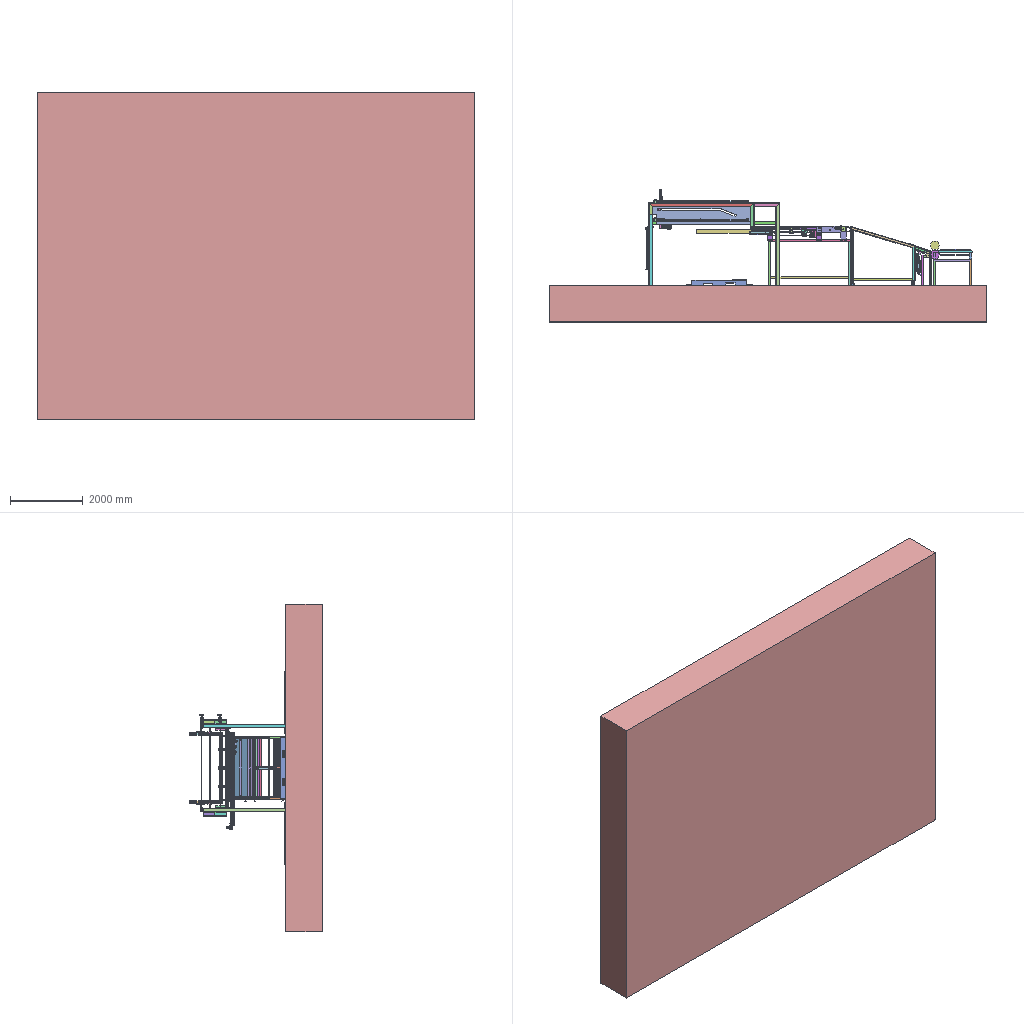Assembly | STEP file | 259 different items | 1357 placed | box 12000 x 3640 x 9000 mm
Parts list (item | name | quantity | parent item | size | volume):
1 | 200W right-angle motor | x3 | in Chuan-type roller line | 116.75 x 104.5 x 320.75 mm | 2722546 mm3
2 | 40 x 40 x 1200-2 | x2 | in FZC-000-001 Upper 1 | 40 x 40 x 1520 mm | 812891 mm3
3 | 40 x 40 x 1700 | x1 | in FZC-000-001 Upper 1 | 40 x 40 x 1620 mm | 866370 mm3
4 | 40 x 40 x 200 | x2 | in FZC-000-001 Upper 1 | 40 x 40 x 98 mm | 52410 mm3
5 | 40 x 40 x 920 | x2 | in FZC-000-001 Upper 1 | 40 x 40 x 1480 mm | 791499 mm3
6 | 40 x 60 x 710 -2_Default<Machined> | x2 | in FZC-000-001 Upper 1 | 710 x 40 x 60 mm | 494666 mm3
7 | 40 x 60 x 940_Default<Machined> | x2 | in FZC-000-001 Upper 1, TN-NHGJQJ-001 | 940 x 40 x 60 mm | 663437 mm3
8 | 40X35X65 oil-free bushing | x4 | in Hydraulic lifting platform assembly | 40 x 40 x 65 mm | 19085 mm3
9 | - | x1 | in MFBR060-L1-14-50-70-M4-33.STEP.STEP_3.STEP_1.STEP_2.STEP.STEP | 29 x 65.5 x 65.5 mm | 78909 mm3
10 | Aluminium profile frame 2_Default<Machined> | x1 | in Sheet stacking line | 2080 x 80 x 40 mm | 1541424 mm3
11 | Aluminium profile frame_Default<Machined> | x1 | in Sheet stacking line | 1808 x 80 x 40 mm | 1339853 mm3
12 | Anti-vibration sleeve | x1 | in Telescopic belt | 173 x 110 x 10 mm | 116462 mm3
13 | BABR060_X2_8f9351658f74_X0_-14.STEP | x1 | in MFBR060-L2-14-50-70-M5-33.STEP | 20 x 20 x 29 mm | 3932 mm3
14 | - | x6 | in GRM4TS-6-75-75-LAA-B10-CLOSED | 156.007 x 55.626 x 50.292 mm | 208315 mm3
15 | BT2022003-01-04 Pin shaft A | x4 | in Hydraulic lifting platform assembly | 109.5 x 31 x 31 mm | 54297 mm3
16 | BT2022003-01-05 Scissor beam A_Default<Machined> | x1 | in Hydraulic lifting platform assembly | 1300 x 120 x 1590 mm | 10641393 mm3
17 | BT2022003-01-06 Scissor beam B_Default<Machined> | x1 | in Hydraulic lifting platform assembly | 1311 x 120 x 1590 mm | 5354127 mm3
18 | BT2022003-01-09 Pin shaft C | x4 | in Hydraulic lifting platform assembly | 125 x 42 x 42 mm | 110638 mm3
19 | BT2022003-01-10 Guide wheel A | x2 | in Hydraulic lifting platform assembly | 26 x 106 x 106 mm | 151941 mm3
20 | BT2022003-10 Liner plate | x4 | in Hydraulic lifting platform assembly | 500 x 4 x 50 mm | 96702 mm3
21 | Baffle 3 | x5 | in Sheet stacking line | 2070 x 50 x 90 mm | 281521 mm3
22 | Base plate 1_Default<Machined> | x1 | in Flip clamping mechanism | 140 x 180 x 12 mm | 295903 mm3
23 | Base plate 2_Default<Machined> | x1 | in Flip clamping mechanism | 40 x 180 x 12 mm | 81882 mm3
24 | Base_Default<Machined> | x1 | in Sheet stacking line | 840 x 60 x 1700 mm | 2443992 mm3
25 | Bearing housing 1 | x3 | in Telescopic belt | 97 x 97 x 35 mm | 155576 mm3
26 | Bearing housing 2 | x3 | in Bearing housing 2 assembly | 114 x 62 x 31 mm | 91139 mm3
27 | Belt | x1 | in Sheet stacking line | 2560 x 1600 x 60 mm | 33125947 mm3
28 | Bracket_Default<Machined> | x2 | in Sheet stacking line | 3700 x 200 x 2275 mm | 12653736 mm3
29 | Connecting plate | x3 | in Telescopic belt | 150 x 240 x 12 mm | 410487 mm3
30 | Conveyor belt | x1 | in Telescopic belt | 2753 x 173 x 1600 mm | 42849624 mm3
31 | Conveyor line bracket_Default<Machined> | x1 | in Sheet stacking line | 1782 x 1478 x 1726 mm | 68319055 mm3
32 | Cross beam 2_Default<Machined> | x2 | in Sheet stacking line | 3400 x 100 x 180 mm | 5412412 mm3
33 | Cross beam_Default<Machined> | x1 | in Sheet stacking line | 2220 x 107.726 x 177.73 mm | 3150772 mm3
34 | DCL01-D40-B-d16-e16 | x1 | in Flip clamping mechanism | 40 x 40 x 66 mm | 65701 mm3
35 | Drive belt | x1 | in Telescopic belt | 332.993 x 128 x 25 mm | 76914 mm3
36 | Drive shaft | x6 | in Chuan-type roller line | 870 x 25 x 25 mm | 420131 mm3
37 | Driving pulley | x4 | in Telescopic belt | 65.94 x 65.413 x 30 mm | 79962 mm3
38 | Driving shaft key | x1 | in Telescopic belt | 30 x 8 x 7 mm | 1584 mm3
39 | EE_SX951P_W | x2 | in Flip clamping mechanism | 13.4 x 12 x 22 mm | 1092 mm3
40 | Edge guard | x6 | in Chuan-type roller line | 35 x 25 x 1700 mm | 453852 mm3
41 | Elastic block | x6 | in Telescopic belt | 24 x 24 x 25 mm | 8627 mm3
42 | End strip | x2 | in Telescopic belt | 10 x 10 x 432 mm | 42976 mm3
43 | FZC-000-002 Rotating shaft A | x4 | in FZC-000-001 Upper 1, Sheet stacking line | 40 x 50 x 100 mm | 133744 mm3
44 | FZC-000-003 Upper cylinder support | x6 | in FZC-000-001 Upper 1, Sheet stacking line | 100 x 60 x 70 mm | 117991 mm3
45 | Fixing block | x2 | in Middle section assembly, Telescopic belt | 105 x 80 x 80 mm | 486425 mm3
46 | Flip baffle_Default<Machined> | x1 | in Sheet stacking line | 1040 x 45 x 1590 mm | 10479554 mm3
47 | Frame 1_Default<Machined> | x2 | in Final assembly | 1700 x 320 x 60 mm | 1222260 mm3
48 | GB893.2-86 internal retaining ring type B 62 | x4 | in Hydraulic lifting platform assembly | 66.2 x 64.58 x 2 mm | 1598 mm3
49 | GB894.2-86 shaft retaining ring type B 25 | x4 | in Hydraulic lifting platform assembly | 28.2 x 30.934 x 1.2 mm | 273.026 mm3
50 | GB894.2-86 shaft retaining ring type B 30 | x4 | in Hydraulic lifting platform assembly | 33.5 x 36.623 x 1.2 mm | 375.357 mm3
51 | GB/T276-94 deep groove ball bearing 6206-2Z | x4 | in Hydraulic lifting platform assembly | 16 x 62 x 62 mm | 23194 mm3
52 | GB/T41-20001 hex nut grade C M12 | x2 | in Sheet stacking line | 19.85 x 17.191 x 12.2 mm | 1737 mm3
53 | GB/T6172.1-2000 hex thin nut grade A and B (M27) | x8 | in Hydraulic lifting platform assembly | 39.233 x 45.2 x 13.5 mm | 9913 mm3
54 | GB/T6172.1-2000 hex thin nut grade A and B M30 | x4 | in Hydraulic lifting platform assembly | 44.137 x 50.85 x 15 mm | 14200 mm3
55 | GDT40-2000 | x3 | in Chuan-type roller line | 20 x 10 x 1400 mm | 237664 mm3
56 | GRM4_B10_BODYOPTION_M | x6 | in GRM4TS-6-75-75-LAA-B10-CLOSED | 50.292 x 55.27 x 73.66 mm | 161375 mm3
57 | GRM4_B10_TUBE_M_71195-001-002100 | x6 | in GRM4TS-6-75-75-LAA-B10-CLOSED | 53.34 x 6.35 x 6.35 mm | 997.325 mm3
58 | GRM4_BREATHER_VENT_71996_M | x6 | in GRM4TS-6-75-75-LAA-B10-CLOSED | 14 x 13 x 15.011 mm | 1457 mm3
59 | GRM4_IMP_PLATE_64636-02_M | x12 | in GRM4TS-6-75-75-LAA-B10-CLOSED | 101.954 x 130.048 x 2.667 mm | 13683 mm3
60 | Gripper baffle | x2 | in Sheet stacking line | 1420 x 5 x 50 mm | 355000 mm3
61 | Ground | x1 | in Sheet stacking line | 12000 x 1000 x 9000 mm | 101165700000 mm3
62 | Guard plate | x144 | in Chuan-type roller line | 328 x 3 x 50 mm | 48733 mm3
63 | Guide rail sliding pair | x3 | in Middle section assembly, Telescopic belt | 63 x 74 x 26.5 mm | 70725 mm3
64 | HB362-65 end not tightened, ground flat 0.25 turns 15×50 | x2 | in Sheet stacking line | 17 x 17 x 50.4 mm | 1550 mm3
65 | HGH20_3_AF0 | x2 | in Sheet stacking line | 44 x 25.4 x 77.5 mm | 65768 mm3
66 | HGR20_3_AF0 | x1 | in Sheet stacking line | 20 x 17.5 x 900 mm | 257708 mm3
67 | HI_BMH070 Flansch | x2 | in Frame-type span dual-rail module | 48.5 x 70.1 x 70 mm | 191060 mm3
68 | Head plate 1 | x1 | in Telescopic belt | 810 x 379.049 x 14 mm | 2266923 mm3
69 | Head plate 2 | x1 | in Telescopic belt | 810 x 160 x 14 mm | 1785161 mm3
70 | Hydraulic cylinder A-400 | x5 | in Final assembly, Sheet stacking line | 60 x 60 x 540 mm | 1442964 mm3
71 | Hydraulic cylinder B-500 | x5 | in Final assembly, Sheet stacking line | 30 x 30 x 411 mm | 278111 mm3
72 | Hydraulic cylinder body SLDPRT | x2 | in 95x80x40x400 hydraulic cylinder assembly | 127.5 x 520 x 95 mm | 2648079 mm3
73 | Idler roller shaft | x1 | in Telescopic belt | 35 x 35 x 408 mm | 356727 mm3
74 | Inner slide strip | x2 | in Telescopic belt | 20 x 20 x 520 mm | 207468 mm3
75 | JB/T7940.1-1995 straight-through grease cup 6 | x2 | in Hydraulic lifting platform assembly | 8 x 13 x 9.238 mm | 360.504 mm3
76 | KFL005 | x6 | in Chuan-type roller line | 60 x 100 x 24.5 mm | 44047 mm3
77 | Key 2 | x1 | in Telescopic belt | 40 x 12 x 8 mm | 3593 mm3
78 | L40 angle steel | x3 | in Telescopic belt | 40 x 40 x 20 mm | 4347 mm3
79 | LEB23-20 | x5 | in Manual lead screw mechanism | 95 x 58 x 61 mm | 169444 mm3
80 | LEB31-20 | x5 | in Manual lead screw mechanism | 95 x 58 x 26 mm | 76469 mm3
81 | Large pulley | x1 | in Telescopic belt | 120.932 x 120.932 x 40 mm | 261557 mm3
82 | Linear motion ball bearing | x4 | in Telescopic belt | 44 x 44 x 44 mm | 35802 mm3
83 | M4_4.STEP_1.STEP_2.STEP.STEP | x4 | in MFBR060-L1-14-50-70-M4-33.STEP_7.STEP_2.STEP.STEP | 24 x 7 x 7 mm | 386.258 mm3
84 | M5.STEP | x1 | in MFBR060-L2-14-50-70-M5-33.STEP | 25 x 8.5 x 8.5 mm | 634.487 mm3
85 | MET_JAW_STD_ROT_GRM4 | x12 | in GRM4TS-6-75-75-LAA-B10-CLOSED | 152.146 x 76.2 x 25.425 mm | 65062 mm3
86 | Main motor | x1 | in Telescopic belt | 120 x 120 x 170 mm | 887990 mm3
87 | Middle plate 1 | x1 | in Telescopic belt | 1500 x 400 x 84 mm | 3461326 mm3
88 | Middle plate 2 | x1 | in Middle section assembly | 1500 x 400 x 84 mm | 3459743 mm3
89 | Mirror HGH20_3_AF0 | x2 | in Sheet stacking line | 44 x 25.4 x 77.5 mm | 65768 mm3
90 | Mirror HGR20_3_AF0 | x1 | in Sheet stacking line | 20 x 17.5 x 900 mm | 257708 mm3
91 | Mirror rail shaft | x1 | in Sheet stacking line | 2134 x 75 x 100 mm | 1735049 mm3
92 | Mirror rail_Default<Machined> | x1 | in Sheet stacking line | 2900 x 115 x 650 mm | 29036229 mm3
93 | Mirror slide plate 2 | x1 | in Sheet stacking line | 90 x 148.62 x 100 mm | 228620 mm3
94 | Mirror slide plate 3 | x1 | in Sheet stacking line | 196 x 218.322 x 100 mm | 404322 mm3
95 | Mirror slider 12 | x1 | in Sheet stacking line | 60 x 60 x 350 mm | 385000 mm3
96 | Mirror slider 13 | x1 | in Sheet stacking line | 60 x 60 x 900 mm | 990000 mm3
97 | Motor bracket | x1 | in Flip clamping mechanism | 65 x 68 x 110 mm | 111617 mm3
98 | Motor mounting plate | x1 | in Telescopic belt | 310 x 180 x 20 mm | 521549 mm3
99 | OT2025004-02-10 Shaft 2 | x1 | in Flip clamping mechanism | 25 x 946 x 25 mm | 439586 mm3
100 | Open CASCADE STEP translator 7.6 56.2.1.1 | x5 | in Open CASCADE STEP translator | 130.4 x 85.907 x 80 mm | 551180 mm3
101 | Open CASCADE STEP translator 7.6 56.2.1.2 | x5 | in Open CASCADE STEP translator | 37.25 x 32.25 x 30.8 mm | 9079 mm3
102 | Open CASCADE STEP translator 7.6 56.2.1.3 | x5 | in Open CASCADE STEP translator | 7.6 x 40.2 x 7.6 mm | 1264 mm3
103 | Open CASCADE STEP translator 7.6 56.2.1.4 | x5 | in Open CASCADE STEP translator | 14.55 x 23.7 x 11.2 mm | 1255 mm3
104 | Open CASCADE STEP translator 7.6 56.2.1.5 | x5 | in Open CASCADE STEP translator | 12.626 x 16.806 x 25 mm | 1310 mm3
105 | Open CASCADE STEP translator 7.6 56.2.1.6 | x5 | in Open CASCADE STEP translator | 6 x 36.756 x 6 mm | 671.876 mm3
106 | Open CASCADE STEP translator 7.6 56.2.1.7 | x5 | in Open CASCADE STEP translator | 19 x 23.7 x 14.5 mm | 1788 mm3
107 | PN59104-114_M_SHCSM6x1x10 | x36 | in GRM4TS-6-75-75-LAA-B10-CLOSED | 10 x 16 x 10 mm | 680.296 mm3
108 | PN59104-141_M_SHCSM8x1.25x25 | x18 | in GRM4TS-6-75-75-LAA-B10-CLOSED | 13 x 33 x 13 mm | 2174 mm3
109 | PN62195-005_METRIC_PLASTIC_TUBE_FITTING | x24 | in GRM4TS-6-75-75-LAA-B10-CLOSED | 26 x 26.85 x 13.856 mm | 3050 mm3
110 | PN_0001-01-01 Lifting platform top cover_Default<Machined> | x1 | in Hydraulic lifting platform assembly | 1500 x 195 x 1800 mm | 133503358 mm3
111 | PN_0001-01-02 Lifting platform base_Default<Machined> | x1 | in Hydraulic lifting platform assembly | 1480 x 1665 x 80 mm | 7503788 mm3
112 | PN_0001-01-07 Pin shaft B | x2 | in Hydraulic lifting platform assembly | 175 x 48.5 x 48.5 mm | 160152 mm3
113 | PN_0001-01-08 Pad | x2 | in Hydraulic lifting platform assembly | 55 x 55 x 5 mm | 8159 mm3
114 | PN_0001-01-11 Guide wheel B | x2 | in Hydraulic lifting platform assembly | 29 x 90 x 90 mm | 98573 mm3
115 | PN_0001-01-12 Sensor board | x1 | in Hydraulic lifting platform assembly | 66 x 58.5 x 2 mm | 7091 mm3
116 | PN_0001-11 Cover plate A | x1 | in Hydraulic lifting platform assembly | 312 x 240 x 3 mm | 222709 mm3
117 | PN_0001-12 Cover plate B | x2 | in Hydraulic lifting platform assembly | 180 x 150 x 340 mm | 329639 mm3
118 | Pad plate | x1 | in FZC-000-001 Upper 1 | 1700 x 1520 x 2 mm | 5168000 mm3
119 | Part 32 | x2 | in Sheet stacking line | 100 x 60 x 40 mm | 240000 mm3
120 | Part 38_Default<Machined> | x1 | in Sheet stacking line | 1720 x 2260 x 1280 mm | 9110278 mm3
121 | Piston rod | x2 | in 95x80x40x400 hydraulic cylinder assembly | 430 x 80 x 80 mm | 691930 mm3
122 | Plain washers-N series-Grade1 A GB_GB_FASTENER_WASHER_PWNA 20 | x3 | in Telescopic belt | 37 x 37 x 3 mm | 2187 mm3
123 | Plate 2 | x6 | in Sheet stacking line | 350 x 5 x 1500 mm | 2625000 mm3
124 | Pressure plate | x7 | in Telescopic belt | 30 x 30 x 6 mm | 3958 mm3
125 | Pressure plate 2 | x66 | in Sheet stacking line | 50 x 6 x 30 mm | 6094 mm3
126 | Pressure plate 3 | x4 | in Sheet stacking line | 1420 x 20 x 30 mm | 852000 mm3
127 | Profile 4060100 | x5 | in TN-NHGJQJ-001 | 40 x 60 x 99.7 mm | 57095 mm3
128 | Profile 40601120 | x1 | in FZC-000-001 Upper 1 | 40 x 60 x 1120 mm | 641390 mm3
129 | Profile 40601200-1 | x4 | in FZC-000-001 Upper 1, TN-NHGJQJ-001 | 40 x 60 x 1200 mm | 664297 mm3
130 | Profile 40601620 | x3 | in FZC-000-001 Upper 1, TN-NHGJQJ-001 | 40 x 60 x 1620 mm | 927725 mm3
131 | Profile 40601700 | x4 | in FZC-000-001 Upper 1, TN-NHGJQJ-001 | 40 x 60 x 1700 mm | 950632 mm3
132 | Profile 4060920 | x2 | in TN-NHGJQJ-001 | 40 x 60 x 920 mm | 526856 mm3
133 | Rail shaft | x1 | in Sheet stacking line | 2134 x 75 x 100 mm | 1735049 mm3
134 | Rail_Default<Machined> | x1 | in Sheet stacking line | 2900 x 115 x 650 mm | 29036229 mm3
135 | Reducer | x1 | in Telescopic belt | 130 x 170 x 120 mm | 1507884 mm3
136 | Retracting rod | x3 | in Telescopic belt | 30 x 30 x 1045 mm | 737225 mm3
137 | Roller 1 | x1 | in Telescopic belt | 120 x 120 x 570 mm | 928585 mm3
138 | Roller 11 | x1 | in Sheet stacking line | 50 x 1800 x 50 mm | 3218952 mm3
139 | Roller 2 | x4 | in Telescopic belt | 50 x 50 x 350 mm | 233051 mm3
140 | Roller line_Default<Machined> | x1 | in Sheet stacking line | 1152 x 1230 x 1771 mm | 196274753 mm3
141 | Roller sheet metal | x3 | in Chuan-type roller line | 380 x 110 x 1700 mm | 4838420 mm3
142 | Roller sheet metal_Mirror Default | x3 | in Chuan-type roller line | 380 x 110 x 1700 mm | 4838420 mm3
143 | Sensor detection tab | x1 | in Flip clamping mechanism | 20 x 18 x 10 mm | 512.842 mm3
144 | Shaft 2 | x1 | in Telescopic belt | 35 x 35 x 550 mm | 418334 mm3
145 | Shaft 3 | x1 | in Telescopic belt | 35 x 35 x 448 mm | 375515 mm3
146 | Shaft 4 | x2 | in Telescopic belt | 35 x 35 x 470 mm | 385852 mm3
147 | Sheath | x1 | in Telescopic belt | 25.34 x 28.859 x 45 mm | 22979 mm3
148 | Sheet metal 11 | x3 | in Chuan-type roller line | 350 x 75 x 1700 mm | 3328088 mm3
149 | Sheet metal 12 | x6 | in Chuan-type roller line | 245 x 75 x 1620 mm | 2491073 mm3
150 | Short conveyor line_Default<Machined> | x1 | in Sheet stacking line | 474.996 x 192.498 x 1720 mm | 30115690 mm3
151 | Single sprocket roller_08B | x96 | in Chuan-type roller line | 365.5 x 65.419 x 65.772 mm | 961298 mm3
152 | Sleeve | x27 | in Chuan-type roller line | 130 x 60 x 60 mm | 302189 mm3
153 | Slide plate 2 | x1 | in Sheet stacking line | 90 x 148.62 x 100 mm | 228620 mm3
154 | Slide plate 3 | x1 | in Sheet stacking line | 196 x 218.322 x 100 mm | 404322 mm3
155 | Slide rod | x3 | in Middle section assembly, Telescopic belt | 640 x 20 x 17.5 mm | 214573 mm3
156 | Slider | x3 | in Middle section assembly, Telescopic belt | 100 x 155 x 60 mm | 283785 mm3
157 | Slider 12 | x1 | in Sheet stacking line | 60 x 60 x 350 mm | 385000 mm3
158 | Slider 13 | x1 | in Sheet stacking line | 60 x 60 x 900 mm | 990000 mm3
159 | Slider pressure plate | x3 | in Slider pressure plate assembly | 100 x 60 x 8 mm | 42576 mm3
160 | Small pulley | x1 | in Telescopic belt | 59.476 x 59.476 x 25 mm | 54452 mm3
161 | Spacer block | x4 | in Telescopic belt | 20 x 20 x 54 mm | 21404 mm3
162 | Spacer block 22 | x10 | in Sheet stacking line | 95 x 40 x 40 mm | 152000 mm3
163 | Spring lock washers--Normal1 type GB_GB_FASTENER_WASHER_SW 20 | x3 | in Telescopic belt | 31.04 x 31.04 x 5 mm | 1973 mm3
164 | Square block | x3 | in Telescopic belt | 60 x 50 x 50 mm | 104625 mm3
165 | Square tube | x1 | in Telescopic belt | 80 x 80 x 80 mm | 136796 mm3
166 | Stopper | x6 | in Stopper assembly | 50 x 50 x 35 mm | 78331 mm3
167 | Stopper rack 12_Default<Machined> | x1 | in Sheet stacking line | 1700 x 164 x 1145 mm | 2370796 mm3
168 | Stopper rack_Default<Machined> | x1 | in Sheet stacking line | 575 x 40 x 2540 mm | 2334872 mm3
169 | Stud | x2 | in Sheet stacking line | 12 x 120 x 12 mm | 13572 mm3
170 | Support rod | x1 | in Telescopic belt | 20 x 20 x 408 mm | 162668 mm3
171 | Support rod 2 | x3 | in Telescopic belt | 20 x 20 x 380 mm | 150404 mm3
172 | Support sheet metal | x126 | in Chuan-type roller line | 112 x 70 x 20 mm | 9602 mm3
173 | Synchronous driving pulley key | x2 | in Telescopic belt | 20 x 5 x 5 mm | 473.175 mm3
174 | Synchronous key | x1 | in Telescopic belt | 25 x 8 x 7 mm | 1400 mm3
175 | Synchronous motor | x1 | in Telescopic belt | 130 x 130 x 239 mm | 1553555 mm3
176 | Synchronous shaft 1 | x3 | in Telescopic belt | 25 x 25 x 89 mm | 25420 mm3
177 | Synchronous shaft 2 | x2 | in Telescopic belt | 40 x 40 x 486 mm | 415215 mm3
178 | T-BDJ-204 | x2 | in Flip clamping mechanism | 37 x 65 x 127 mm | 102514 mm3
179 | TN-NHGJQJ-001-001 | x4 | in Sheet stacking line, TN-NHGJQJ-001 | 150 x 40 x 55 mm | 96398 mm3
180 | TN-NHGJQJ-001-002 | x6 | in Sheet stacking line, TN-NHGJQJ-001 | 100 x 120 x 110 mm | 222546 mm3
181 | Telescopic plate | x1 | in Telescopic belt | 296 x 35 x 1190 mm | 1170000 mm3
182 | Thin steel plate | x1 | in Telescopic belt | 350 x 1 x 1590 mm | 556500 mm3
183 | Timing belt | x3 | in Telescopic belt | 1001 x 71 x 25 mm | 155522 mm3
184 | Timing pulley | x2 | in Telescopic belt | 65.94 x 65.413 x 30 mm | 80276 mm3
185 | Tray | x1 | in Sheet stacking line | 1500 x 150 x 1700 mm | 287460631 mm3
186 | Underframe_Default<Machined> | x1 | in Sheet stacking line | 1740 x 260 x 970 mm | 7091962 mm3
187 | Unpowered roller | x48 | in Chuan-type roller line | 334.5 x 60 x 60 mm | 930239 mm3
188 | X2MH010A-N2C (connector type) -1 | x1 | in Flip clamping mechanism | 40 x 54.95 x 96 mm | 118411 mm3
189 | YBLX-ME-8108 limit switch | x1 | in Hydraulic lifting platform assembly | 28.5 x 180 x 50 mm | 106221 mm3
190 | _1-LCV02-25-5-L1400-F27-P101 | x5 | in Manual lead screw mechanism | 25 x 25 x 2604 mm | 1237665 mm3
191 | _2-LCV02-25-5-L1400-F27-P102 | x5 | in Manual lead screw mechanism, Sheet stacking line | 48 x 62 x 51 mm | 50671 mm3
192 | _Achsprofil-SBG - PAS42 B 1236 | x4 | in Frame-type span dual-rail module | 2456 x 60 x 60 mm | 8161158 mm3
193 | _BMH070 Abschlussdeckel | x2 | in Frame-type span dual-rail module | 8 x 70 x 70 mm | 28903 mm3
194 | _BMH070 Lagerschild2A154 | x2 | in Frame-type span dual-rail module | 100 x 70.1 x 70 mm | 431023 mm3
195 | _BMH070 Signalstecker gerade1 | x2 | in Frame-type span dual-rail module | 51 x 39.4 x 28 mm | 34337 mm3
196 | _BMH070 Signalstecker gerade2 | x2 | in Frame-type span dual-rail module | 54 x 39.4 x 28 mm | 35555 mm3
197 | _BMH070 Welle20 | x2 | in Frame-type span dual-rail module | 31.5 x 17 x 17 mm | 3904 mm3
198 | _CEL21-100-P-001 | x4 | in CEL21-100-P | 81.4 x 134 x 162 mm | 463368 mm3
199 | _CEL21-100-P-002 | x4 | in CEL21-100-P | 100 x 10 x 115 mm | 55123 mm3
200 | _Endblock-SBG - PAS42 B 1 | x8 | in Frame-type span dual-rail module | 80 x 74 x 60 mm | 295323 mm3
201 | _F-SE100CB | x1 | - | 61 x 110 x 119 mm | 221745 mm3
202 | _F-SI100CR(SE) | x1 | - | 84 x 90 x 96 mm | 270895 mm3
203 | _Gummipuffer-SBG - PAS42 B | x8 | in Frame-type span dual-rail module | 18 x 16.46 x 59 mm | 11573 mm3
204 | _Hexagon socket head cap screw DIN 912 - M5x16 | x8 | in Frame-type span dual-rail module | 21 x 8.5 x 8.5 mm | 547.668 mm3
205 | _Hexagon socket head cap screw DIN 912 - M5x20 | x8 | in Frame-type span dual-rail module | 25 x 8.5 x 8.5 mm | 626.207 mm3
206 | _IBC23-45-100_002 | x8 | in Sheet stacking line | 60 x 37 x 104.901 mm | 162215 mm3
207 | _IBC23-45-1500_001 | x2 | in Sheet stacking line | 28 x 26 x 2540 mm | 1504984 mm3
208 | _Kupplungsgehaeuse-SBG - PAS42 B | x2 | in Frame-type span dual-rail module | 26 x 60 x 60 mm | 42515 mm3
209 | _L170 - PAS42 B | x8 | in Frame-type span dual-rail module, Sheet stacking line | - | -
210 | _MAX100010001NA0_cupling2 | x8 | in Frame-type span dual-rail module | 61 x 40 x 40 mm | 52985 mm3
211 | _MAX100010001N_rod2 | x4 | in Frame-type span dual-rail module | 2216 x 20 x 20 mm | 695277 mm3
212 | _MoAd-PLE60x-PAS42 B-2 | x2 | in Frame-type span dual-rail module | 30.5 x 62 x 62 mm | 64839 mm3
213 | _PLE60-5_MOTOR(Housing 1-1-3) | x2 | in Frame-type span dual-rail module | 82 x 60 x 60 mm | 141092 mm3
214 | _PLE60-5_MOTOR-OP2 (intermediate flanges 11-23-60-75-5-70-2.5) | x2 | in Frame-type span dual-rail module | 24.2 x 70 x 70 mm | 107278 mm3
215 | _SE-100 CA_CB_CR Screw | x4 | - | 33 x 13 x 13 mm | 2886 mm3
216 | _SE-100-M20x1.5 - Nut | x1 | - | 10 x 30.022 x 26 mm | 3125 mm3
217 | _SE-100x300-CR (0) | x1 | - | 478 x 110 x 110 mm | 2351296 mm3
218 | _SE-100x300-CR(0)_r | x1 | - | 482 x 98.6 x 98.6 mm | 543204 mm3
219 | _Schaltwinkel l170-SBG - PAS42 B | x2 | in Frame-type span dual-rail module | 170 x 11 x 15 mm | 5664 mm3
220 | _Sensor SBG - PAS42 B -1 | x4 | in Frame-type span dual-rail module | 17.5 x 37 x 23 mm | 3611 mm3
221 | _X2_4e007ea751859f7f5708_X0_MFB060_2.STEP.STEP | x1 | in MFBR060-L2-14-50-70-M4-33.STEP.STEP | 65.5 x 29 x 65.5 mm | 84346 mm3
222 | _X2_6cb95c01_X0_20X30X4_5.STEP.STEP | x1 | in MFBR060-L2-14-50-70-M4-33.STEP.STEP | 3.6 x 30.624 x 30.624 mm | 1217 mm3
223 | _X2_8c0365745957_X0_14-8 | x1 | in MFBR060-L2-8-30-46-M4-33 | 18 x 16.485 x 16.5 mm | 1831 mm3
224 | _X2_8f9351656cd55170_X0_MAB060-30-46-M4 | x1 | in MFBR060-L2-8-30-46-M4-33 | 60 x 23 x 60 mm | 47434 mm3
225 | _X2_8f9351657aef58f34f53_X0_MABR060.STEP_3.STEP_1.STEP_2.STEP.STEP | x1 | in MFBR060-L1-14-50-70-M4-33.STEP_5.STEP_1.STEP_2.STEP.STEP | 60 x 60 x 19.5 mm | 47406 mm3
226 | _X2_8f9351fa51859f7f5708_X0_MFB060_5.STEP.STEP | x1 | in MFBR060-L2-14-50-70-M4-33.STEP.STEP | 43 x 65.5 x 65.5 mm | 50980 mm3
227 | _X2_8f9351fa884c661f67b6_X0_MAB060-16X28.5XM5_2.STEP.STEP | x1 | in MFBR060-L2-14-50-70-M4-33.STEP.STEP | 38 x 20 x 20 mm | 8651 mm3
228 | _X2_8f9351fa95017d2773af_X0_MAB060_5.STEP.STEP | x1 | in MFBR060-L2-14-50-70-M4-33.STEP.STEP | 43 x 6 x 43 mm | 4269 mm3
229 | _X2_95017d2773af_X0_MAB060-14.STEP | x1 | in MFBR060-L2-14-50-70-M5-33.STEP | 36.973 x 12 x 37 mm | 8292 mm3
230 | - | x1 | in MFBR060-L1-14-50-70-M4-33.STEP.STEP_3.STEP_1.STEP_2.STEP.STEP | - | -
231 | circlips for holes--type a gb_GB_CONNECTING_PIECE_RING_RRH 45 | x4 | in Telescopic belt | 48.5 x 46.654 x 1.5 mm | 718.222 mm3
232 | circlips for shaft--type b gb_GB_CONNECTING_PIECE_RINGS_CSB 30 | x8 | in Telescopic belt | 33.5 x 36.621 x 1.2 mm | 375.469 mm3
233 | hex head bolts-full thread grade c gb_GB_FASTENER_BOLT_HHBFTC M10X30-S | x9 | in Telescopic belt | 36.4 x 18.475 x 16 mm | 3743 mm3
234 | hex head bolts-full thread grade c gb_GB_FASTENER_BOLT_HHBFTC M12X30-S | x24 | in Bearing housing 2 assembly, Telescopic belt | 37.5 x 20.785 x 18 mm | 5456 mm3
235 | hex head bolts-full thread grade c gb_GB_FASTENER_BOLT_HHBFTC M16X90-S | x1 | in Telescopic belt | 100 x 27.713 x 24 mm | 22987 mm3
236 | hex head bolts-full thread grade c gb_GB_FASTENER_BOLT_HHBFTC M6X12-S | x8 | in Telescopic belt | 16 x 11.547 x 10 mm | 674.444 mm3
237 | hex head bolts-full thread grade c gb_GB_FASTENER_BOLT_HHBFTC M6X16-S | x5 | in Telescopic belt | 20 x 11.547 x 10 mm | 787.542 mm3
238 | hex head bolts-full thread grade c gb_GB_FASTENER_BOLT_HHBFTC M6X20-S | x8 | in Telescopic belt | 24 x 11.547 x 10 mm | 900.64 mm3
239 | hex head bolts-full thread grade c gb_GB_FASTENER_BOLT_HHBFTC M6X25-S | x2 | in Telescopic belt | 29 x 11.547 x 10 mm | 1042 mm3
240 | hex head bolts-full thread grade c gb_GB_FASTENER_BOLT_HHBFTC M6X30-S | x2 | in Telescopic belt | 34 x 11.547 x 10 mm | 1183 mm3
241 | hex head bolts-full thread grade c gb_GB_FASTENER_BOLT_HHBFTC M6X50-S | x3 | in Telescopic belt | 54 x 11.547 x 10 mm | 1749 mm3
242 | hex head bolts-full thread grade c gb_GB_FASTENER_BOLT_HHBFTC M8X25-S | x4 | in Telescopic belt | 30.3 x 15.011 x 13 mm | 2010 mm3
243 | hex head bolts-full thread grade c gb_GB_FASTENER_BOLT_HHBFTC M8X35-S | x4 | in Telescopic belt | 40.3 x 15.011 x 13 mm | 2512 mm3
244 | hex nuts, style 1-grades ab gb_GB_FASTENER_NUT_SNAB1 B M20-N | x3 | in Telescopic belt | 34.641 x 30 x 18 mm | 9644 mm3
245 | hex nuts, style 1-grades ab gb_GB_FASTENER_NUT_SNAB1 M16-N | x1 | in Telescopic belt | 27.713 x 24 x 14.8 mm | 5071 mm3
246 | hex nuts, style 1-grades ab gb_GB_FASTENER_NUT_SNAB1 M4-N | x10 | in Telescopic belt | 8.083 x 7 x 3.2 mm | 104.298 mm3
247 | hex nuts, style 1-grades ab gb_GB_FASTENER_NUT_SNAB1 M6-N | x4 | in Telescopic belt | 11.547 x 10 x 5.2 mm | 340.663 mm3
248 | hexagon socket head cap screws gb_GB_FASTENER_SCREWS_HSHCS M4X20-N | x2 | in Telescopic belt | 24 x 7 x 7 mm | 386.259 mm3
249 | hexagon socket head cap screws gb_GB_FASTENER_SCREWS_HSHCS M4X40-N | x3 | in Telescopic belt | 44 x 7 x 7 mm | 637.59 mm3
250 | hexagon socket head cap screws gb_GB_FASTENER_SCREWS_HSHCS M6X20-N | x11 | in Middle section assembly | 26 x 10 x 10 mm | 958.106 mm3
251 | hexagon socket head cap screws gb_GB_FASTENER_SCREWS_HSHCS M6X35-N | x24 | in Stopper assembly | 41 x 10 x 10 mm | 1382 mm3
252 | hexagon socket head cap screws gb_GB_FASTENER_SCREWS_HSHCS M6X50-N | x2 | in Telescopic belt | 56 x 10 x 10 mm | 1806 mm3
253 | hexagon socket head cap screws gb_GB_FASTENER_SCREWS_HSHCS M6X55-N | x2 | in Telescopic belt | 61 x 10 x 10 mm | 1948 mm3
254 | hexagon socket head cap screws gb_GB_FASTENER_SCREWS_HSHCS M6X60-N | x3 | in Telescopic belt | 66 x 10 x 10 mm | 2089 mm3
255 | hexagon socket head cap screws gb_GB_FASTENER_SCREWS_HSHCS M8X20-N | x4 | in Telescopic belt | 28 x 13 x 13 mm | 1916 mm3
256 | hexagon socket head cap screws gb_GB_FASTENER_SCREWS_HSHCS M8X70-N | x6 | in Middle section assembly, Telescopic belt | 78 x 13 x 13 mm | 4429 mm3
257 | radial ball bearing_68_skf_SKF - 61906 - 18,SI,NC,18_68 | x8 | in Telescopic belt | 9 x 47 x 47 mm | 7474 mm3
258 | short pitch roller chain wheel_s_iso_Chain wheel ISO - 14Z 08A-1 --14SB75H20L20.0S1 | x3 | in Chuan-type roller line | 20.001 x 63.542 x 65.028 mm | 28318 mm3
259 | short pitch roller chain wheel_s_iso_Chain wheel ISO - 14Z 08A-1 --14SB75H20L22.0R1 | x3 | in Chuan-type roller line | 20.001 x 63.542 x 65.028 mm | 26785 mm3